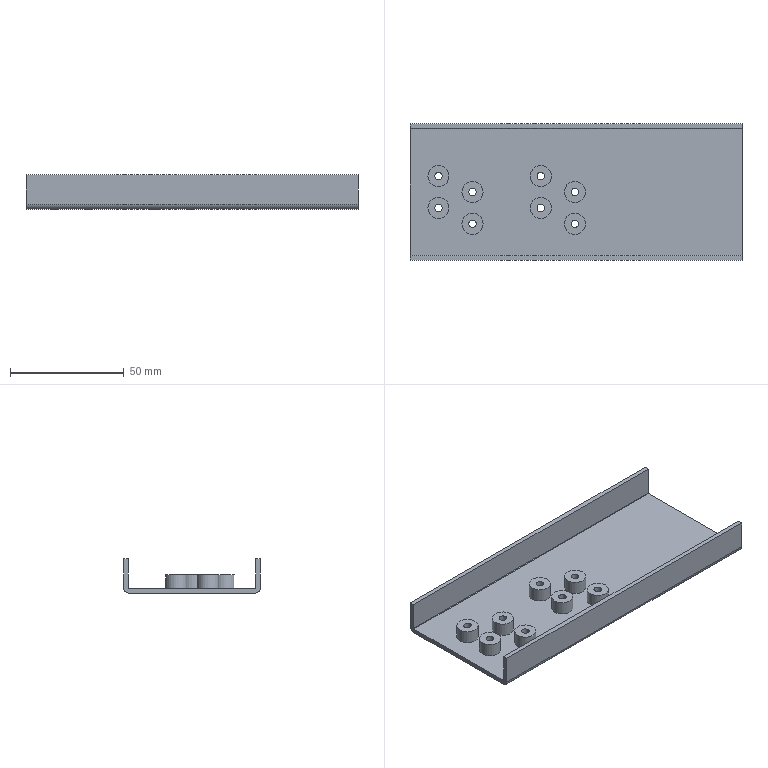Part | STEP file | FHD-021-001-Y rack welded part Y | 1 solid | 38 faces | box 146 x 60 x 15 mm | volume 27524 mm3 | cylinder 20 | plane 18 | commonest cylinder face diameters 3.3 x8 9.3 x8 0.4 x2 4.4 x2